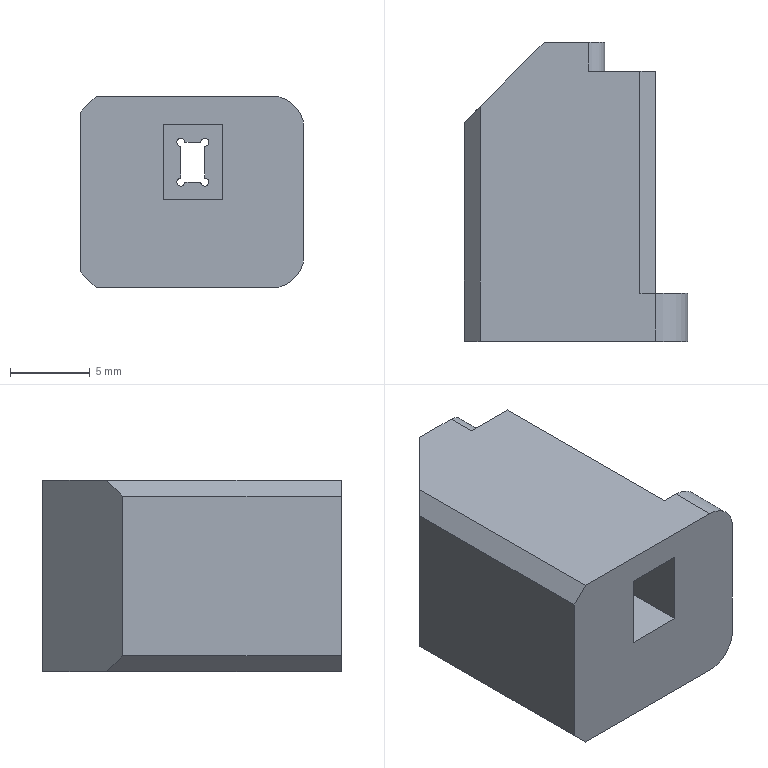Part | STEP file | 03-02 left cutter pad block | 1 solid | 40 faces | box 14 x 18.7 x 12 mm | volume 2273 mm3 | plane 26 | cylinder 14 | commonest cylinder face diameters 0.5 x6 0.6 x4 2 x2 4 x2
STEP:
#1=CARTESIAN_POINT('',(2.4,16.7,-0.58));
#2=VERTEX_POINT('',#1);
#3=CARTESIAN_POINT('',(2.4,16.7,0.02));
#4=VERTEX_POINT('',#3);
#5=CARTESIAN_POINT('',(2.4,16.7,-0.28));
#6=DIRECTION('',(0.,1.,0.));
#7=DIRECTION('',(0.,0.,1.));
#8=AXIS2_PLACEMENT_3D('',#5,#6,#7);
#9=CIRCLE('',#8,0.3);
#10=EDGE_CURVE('',#2,#4,#9,.T.);
#11=ORIENTED_EDGE('',*,*,#10,.F.);
#12=CARTESIAN_POINT('',(2.4,18.7,-0.58));
#13=VERTEX_POINT('',#12);
#14=CARTESIAN_POINT('',(2.4,16.7,-0.58));
#15=DIRECTION('',(0.,1.,0.));
#16=VECTOR('',#15,1000.);
#17=LINE('',#14,#16);
#18=EDGE_CURVE('',#2,#13,#17,.T.);
#19=ORIENTED_EDGE('',*,*,#18,.T.);
#20=CARTESIAN_POINT('',(2.4,18.7,0.02));
#21=VERTEX_POINT('',#20);
#22=CARTESIAN_POINT('',(2.4,18.7,-0.28));
#23=DIRECTION('',(0.,1.,0.));
#24=DIRECTION('',(0.,0.,1.));
#25=AXIS2_PLACEMENT_3D('',#22,#23,#24);
#26=CIRCLE('',#25,0.3);
#27=EDGE_CURVE('',#13,#21,#26,.T.);
#28=ORIENTED_EDGE('',*,*,#27,.T.);
#29=CARTESIAN_POINT('',(2.4,16.7,0.02));
#30=DIRECTION('',(0.,1.,0.));
#31=VECTOR('',#30,1000.);
#32=LINE('',#29,#31);
#33=EDGE_CURVE('',#4,#21,#32,.T.);
#34=ORIENTED_EDGE('',*,*,#33,.F.);
#35=EDGE_LOOP('',(#11,#19,#28,#34));
#36=FACE_OUTER_BOUND('',#35,.T.);
#37=CARTESIAN_POINT('',(2.4,16.7,-0.28));
#38=DIRECTION('',(0.,1.,0.));
#39=DIRECTION('',(0.,0.,1.));
#40=AXIS2_PLACEMENT_3D('',#37,#38,#39);
#41=CYLINDRICAL_SURFACE('',#40,0.3);
#42=ADVANCED_FACE('',(#36),#41,.F.);
#43=CARTESIAN_POINT('',(2.4,16.7,0.62));
#44=VERTEX_POINT('',#43);
#45=CARTESIAN_POINT('',(2.4,16.7,1.22));
#46=VERTEX_POINT('',#45);
#47=CARTESIAN_POINT('',(2.4,16.7,0.92));
#48=DIRECTION('',(0.,1.,0.));
#49=DIRECTION('',(0.,0.,1.));
#50=AXIS2_PLACEMENT_3D('',#47,#48,#49);
#51=CIRCLE('',#50,0.3);
#52=EDGE_CURVE('',#44,#46,#51,.T.);
#53=ORIENTED_EDGE('',*,*,#52,.F.);
#54=CARTESIAN_POINT('',(2.4,18.7,0.62));
#55=VERTEX_POINT('',#54);
#56=CARTESIAN_POINT('',(2.4,16.7,0.62));
#57=DIRECTION('',(0.,1.,0.));
#58=VECTOR('',#57,1000.);
#59=LINE('',#56,#58);
#60=EDGE_CURVE('',#44,#55,#59,.T.);
#61=ORIENTED_EDGE('',*,*,#60,.T.);
#62=CARTESIAN_POINT('',(2.4,18.7,1.22));
#63=VERTEX_POINT('',#62);
#64=CARTESIAN_POINT('',(2.4,18.7,0.92));
#65=DIRECTION('',(0.,1.,0.));
#66=DIRECTION('',(0.,0.,1.));
#67=AXIS2_PLACEMENT_3D('',#64,#65,#66);
#68=CIRCLE('',#67,0.3);
#69=EDGE_CURVE('',#55,#63,#68,.T.);
#70=ORIENTED_EDGE('',*,*,#69,.T.);
#71=CARTESIAN_POINT('',(2.4,16.7,1.22));
#72=DIRECTION('',(0.,1.,0.));
#73=VECTOR('',#72,1000.);
#74=LINE('',#71,#73);
#75=EDGE_CURVE('',#46,#63,#74,.T.);
#76=ORIENTED_EDGE('',*,*,#75,.F.);
#77=EDGE_LOOP('',(#53,#61,#70,#76));
#78=FACE_OUTER_BOUND('',#77,.T.);
#79=CARTESIAN_POINT('',(2.4,16.7,0.92));
#80=DIRECTION('',(0.,1.,0.));
#81=DIRECTION('',(0.,0.,1.));
#82=AXIS2_PLACEMENT_3D('',#79,#80,#81);
#83=CYLINDRICAL_SURFACE('',#82,0.3);
#84=ADVANCED_FACE('',(#78),#83,.F.);
#85=CARTESIAN_POINT('',(1.8,12.,2.87));
#86=VERTEX_POINT('',#85);
#87=CARTESIAN_POINT('',(1.8,12.,3.37));
#88=VERTEX_POINT('',#87);
#89=CARTESIAN_POINT('',(1.8,12.,3.12));
#90=DIRECTION('',(0.,-1.,0.));
#91=DIRECTION('',(0.,0.,-1.));
#92=AXIS2_PLACEMENT_3D('',#89,#90,#91);
#93=CIRCLE('',#92,0.25);
#94=EDGE_CURVE('',#86,#88,#93,.T.);
#95=ORIENTED_EDGE('',*,*,#94,.T.);
#96=CARTESIAN_POINT('',(1.8,18.7,3.37));
#97=VERTEX_POINT('',#96);
#98=CARTESIAN_POINT('',(1.8,8.7,3.37));
#99=DIRECTION('',(0.,1.,0.));
#100=VECTOR('',#99,1000.);
#101=LINE('',#98,#100);
#102=EDGE_CURVE('',#88,#97,#101,.T.);
#103=ORIENTED_EDGE('',*,*,#102,.T.);
#104=CARTESIAN_POINT('',(1.8,18.7,2.87));
#105=VERTEX_POINT('',#104);
#106=CARTESIAN_POINT('',(1.8,18.7,3.12));
#107=DIRECTION('',(0.,1.,0.));
#108=DIRECTION('',(0.,0.,1.));
#109=AXIS2_PLACEMENT_3D('',#106,#107,#108);
#110=CIRCLE('',#109,0.25);
#111=EDGE_CURVE('',#97,#105,#110,.T.);
#112=ORIENTED_EDGE('',*,*,#111,.T.);
#113=CARTESIAN_POINT('',(1.8,8.7,2.87));
#114=DIRECTION('',(0.,1.,0.));
#115=VECTOR('',#114,1000.);
#116=LINE('',#113,#115);
#117=EDGE_CURVE('',#86,#105,#116,.T.);
#118=ORIENTED_EDGE('',*,*,#117,.F.);
#119=EDGE_LOOP('',(#95,#103,#112,#118));
#120=FACE_OUTER_BOUND('',#119,.T.);
#121=CARTESIAN_POINT('',(1.8,8.7,3.12));
#122=DIRECTION('',(0.,1.,0.));
#123=DIRECTION('',(0.,0.,1.));
#124=AXIS2_PLACEMENT_3D('',#121,#122,#123);
#125=CYLINDRICAL_SURFACE('',#124,0.25);
#126=ADVANCED_FACE('',(#120),#125,.F.);
#127=CARTESIAN_POINT('',(0.55,12.,3.12));
#128=VERTEX_POINT('',#127);
#129=CARTESIAN_POINT('',(0.3,12.,3.37));
#130=VERTEX_POINT('',#129);
#131=CARTESIAN_POINT('',(0.3,12.,3.12));
#132=DIRECTION('',(0.,-1.,0.));
#133=DIRECTION('',(0.,0.,-1.));
#134=AXIS2_PLACEMENT_3D('',#131,#132,#133);
#135=CIRCLE('',#134,0.25);
#136=EDGE_CURVE('',#128,#130,#135,.T.);
#137=ORIENTED_EDGE('',*,*,#136,.T.);
#138=CARTESIAN_POINT('',(0.3,18.7,3.37));
#139=VERTEX_POINT('',#138);
#140=CARTESIAN_POINT('',(0.3,8.7,3.37));
#141=DIRECTION('',(0.,1.,0.));
#142=VECTOR('',#141,1000.);
#143=LINE('',#140,#142);
#144=EDGE_CURVE('',#130,#139,#143,.T.);
#145=ORIENTED_EDGE('',*,*,#144,.T.);
#146=CARTESIAN_POINT('',(0.55,18.7,3.12));
#147=VERTEX_POINT('',#146);
#148=CARTESIAN_POINT('',(0.3,18.7,3.12));
#149=DIRECTION('',(0.,1.,0.));
#150=DIRECTION('',(0.,0.,1.));
#151=AXIS2_PLACEMENT_3D('',#148,#149,#150);
#152=CIRCLE('',#151,0.25);
#153=EDGE_CURVE('',#139,#147,#152,.T.);
#154=ORIENTED_EDGE('',*,*,#153,.T.);
#155=CARTESIAN_POINT('',(0.55,8.7,3.12));
#156=DIRECTION('',(0.,1.,0.));
#157=VECTOR('',#156,1000.);
#158=LINE('',#155,#157);
#159=EDGE_CURVE('',#128,#147,#158,.T.);
#160=ORIENTED_EDGE('',*,*,#159,.F.);
#161=EDGE_LOOP('',(#137,#145,#154,#160));
#162=FACE_OUTER_BOUND('',#161,.T.);
#163=CARTESIAN_POINT('',(0.3,8.7,3.12));
#164=DIRECTION('',(0.,1.,0.));
#165=DIRECTION('',(0.,0.,1.));
#166=AXIS2_PLACEMENT_3D('',#163,#164,#165);
#167=CYLINDRICAL_SURFACE('',#166,0.25);
#168=ADVANCED_FACE('',(#162),#167,.F.);
#169=CARTESIAN_POINT('',(0.3,18.7,0.87));
#170=VERTEX_POINT('',#169);
#171=CARTESIAN_POINT('',(0.3,18.7,2.87));
#172=VERTEX_POINT('',#171);
#173=CARTESIAN_POINT('',(0.3,18.7,0.62));
#174=DIRECTION('',(0.,0.,1.));
#175=VECTOR('',#174,1000.);
#176=LINE('',#173,#175);
#177=EDGE_CURVE('',#170,#172,#176,.T.);
#178=ORIENTED_EDGE('',*,*,#177,.T.);
#179=CARTESIAN_POINT('',(0.3,12.,2.87));
#180=VERTEX_POINT('',#179);
#181=CARTESIAN_POINT('',(0.3,8.7,2.87));
#182=DIRECTION('',(0.,-1.,0.));
#183=VECTOR('',#182,1000.);
#184=LINE('',#181,#183);
#185=EDGE_CURVE('',#172,#180,#184,.T.);
#186=ORIENTED_EDGE('',*,*,#185,.T.);
#187=CARTESIAN_POINT('',(0.3,12.,0.87));
#188=VERTEX_POINT('',#187);
#189=CARTESIAN_POINT('',(0.3,12.,0.62));
#190=DIRECTION('',(0.,0.,1.));
#191=VECTOR('',#190,1000.);
#192=LINE('',#189,#191);
#193=EDGE_CURVE('',#188,#180,#192,.T.);
#194=ORIENTED_EDGE('',*,*,#193,.F.);
#195=CARTESIAN_POINT('',(0.3,8.7,0.87));
#196=DIRECTION('',(0.,1.,0.));
#197=VECTOR('',#196,1000.);
#198=LINE('',#195,#197);
#199=EDGE_CURVE('',#188,#170,#198,.T.);
#200=ORIENTED_EDGE('',*,*,#199,.T.);
#201=EDGE_LOOP('',(#178,#186,#194,#200));
#202=FACE_OUTER_BOUND('',#201,.T.);
#203=CARTESIAN_POINT('',(0.3,-11.3,0.62));
#204=DIRECTION('',(-1.,0.,0.));
#205=DIRECTION('',(0.,0.,1.));
#206=AXIS2_PLACEMENT_3D('',#203,#204,#205);
#207=PLANE('',#206);
#208=ADVANCED_FACE('',(#202),#207,.F.);
#209=CARTESIAN_POINT('',(1.55,12.,0.62));
#210=VERTEX_POINT('',#209);
#211=CARTESIAN_POINT('',(0.55,12.,0.62));
#212=VERTEX_POINT('',#211);
#213=CARTESIAN_POINT('',(0.3,12.,0.62));
#214=DIRECTION('',(-1.,0.,0.));
#215=VECTOR('',#214,1000.);
#216=LINE('',#213,#215);
#217=EDGE_CURVE('',#210,#212,#216,.T.);
#218=ORIENTED_EDGE('',*,*,#217,.F.);
#219=CARTESIAN_POINT('',(1.55,18.7,0.62));
#220=VERTEX_POINT('',#219);
#221=CARTESIAN_POINT('',(1.55,8.7,0.62));
#222=DIRECTION('',(0.,1.,0.));
#223=VECTOR('',#222,1000.);
#224=LINE('',#221,#223);
#225=EDGE_CURVE('',#210,#220,#224,.T.);
#226=ORIENTED_EDGE('',*,*,#225,.T.);
#227=CARTESIAN_POINT('',(0.55,18.7,0.62));
#228=VERTEX_POINT('',#227);
#229=CARTESIAN_POINT('',(0.3,18.7,0.62));
#230=DIRECTION('',(-1.,0.,0.));
#231=VECTOR('',#230,1000.);
#232=LINE('',#229,#231);
#233=EDGE_CURVE('',#220,#228,#232,.T.);
#234=ORIENTED_EDGE('',*,*,#233,.T.);
#235=CARTESIAN_POINT('',(0.55,8.7,0.62));
#236=DIRECTION('',(0.,-1.,0.));
#237=VECTOR('',#236,1000.);
#238=LINE('',#235,#237);
#239=EDGE_CURVE('',#228,#212,#238,.T.);
#240=ORIENTED_EDGE('',*,*,#239,.T.);
#241=EDGE_LOOP('',(#218,#226,#234,#240));
#242=FACE_OUTER_BOUND('',#241,.T.);
#243=CARTESIAN_POINT('',(0.3,-11.3,0.62));
#244=DIRECTION('',(0.,0.,-1.));
#245=DIRECTION('',(-1.,0.,0.));
#246=AXIS2_PLACEMENT_3D('',#243,#244,#245);
#247=PLANE('',#246);
#248=ADVANCED_FACE('',(#242),#247,.F.);
#249=CARTESIAN_POINT('',(1.8,12.,0.87));
#250=VERTEX_POINT('',#249);
#251=CARTESIAN_POINT('',(1.8,12.,0.62));
#252=DIRECTION('',(0.,0.,-1.));
#253=VECTOR('',#252,1000.);
#254=LINE('',#251,#253);
#255=EDGE_CURVE('',#86,#250,#254,.T.);
#256=ORIENTED_EDGE('',*,*,#255,.F.);
#257=ORIENTED_EDGE('',*,*,#117,.T.);
#258=CARTESIAN_POINT('',(1.8,18.7,0.87));
#259=VERTEX_POINT('',#258);
#260=CARTESIAN_POINT('',(1.8,18.7,0.62));
#261=DIRECTION('',(0.,0.,-1.));
#262=VECTOR('',#261,1000.);
#263=LINE('',#260,#262);
#264=EDGE_CURVE('',#105,#259,#263,.T.);
#265=ORIENTED_EDGE('',*,*,#264,.T.);
#266=CARTESIAN_POINT('',(1.8,8.7,0.87));
#267=DIRECTION('',(0.,-1.,0.));
#268=VECTOR('',#267,1000.);
#269=LINE('',#266,#268);
#270=EDGE_CURVE('',#259,#250,#269,.T.);
#271=ORIENTED_EDGE('',*,*,#270,.T.);
#272=EDGE_LOOP('',(#256,#257,#265,#271));
#273=FACE_OUTER_BOUND('',#272,.T.);
#274=CARTESIAN_POINT('',(1.8,-11.3,0.62));
#275=DIRECTION('',(1.,0.,0.));
#276=DIRECTION('',(0.,0.,-1.));
#277=AXIS2_PLACEMENT_3D('',#274,#275,#276);
#278=PLANE('',#277);
#279=ADVANCED_FACE('',(#273),#278,.F.);
#280=CARTESIAN_POINT('',(1.55,18.7,3.12));
#281=VERTEX_POINT('',#280);
#282=CARTESIAN_POINT('',(0.3,18.7,3.12));
#283=DIRECTION('',(1.,0.,0.));
#284=VECTOR('',#283,1000.);
#285=LINE('',#282,#284);
#286=EDGE_CURVE('',#147,#281,#285,.T.);
#287=ORIENTED_EDGE('',*,*,#286,.T.);
#288=CARTESIAN_POINT('',(1.55,12.,3.12));
#289=VERTEX_POINT('',#288);
#290=CARTESIAN_POINT('',(1.55,8.7,3.12));
#291=DIRECTION('',(0.,-1.,0.));
#292=VECTOR('',#291,1000.);
#293=LINE('',#290,#292);
#294=EDGE_CURVE('',#281,#289,#293,.T.);
#295=ORIENTED_EDGE('',*,*,#294,.T.);
#296=CARTESIAN_POINT('',(0.3,12.,3.12));
#297=DIRECTION('',(1.,0.,0.));
#298=VECTOR('',#297,1000.);
#299=LINE('',#296,#298);
#300=EDGE_CURVE('',#128,#289,#299,.T.);
#301=ORIENTED_EDGE('',*,*,#300,.F.);
#302=ORIENTED_EDGE('',*,*,#159,.T.);
#303=EDGE_LOOP('',(#287,#295,#301,#302));
#304=FACE_OUTER_BOUND('',#303,.T.);
#305=CARTESIAN_POINT('',(0.3,-11.3,3.12));
#306=DIRECTION('',(0.,0.,1.));
#307=DIRECTION('',(1.,0.,0.));
#308=AXIS2_PLACEMENT_3D('',#305,#306,#307);
#309=PLANE('',#308);
#310=ADVANCED_FACE('',(#304),#309,.F.);
#311=CARTESIAN_POINT('',(6.,3.,-5.));
#312=VERTEX_POINT('',#311);
#313=CARTESIAN_POINT('',(6.,3.,5.));
#314=VERTEX_POINT('',#313);
#315=CARTESIAN_POINT('',(6.,3.,-6.));
#316=DIRECTION('',(0.,0.,1.));
#317=VECTOR('',#316,1000.);
#318=LINE('',#315,#317);
#319=EDGE_CURVE('',#312,#314,#318,.T.);
#320=ORIENTED_EDGE('',*,*,#319,.F.);
#321=CARTESIAN_POINT('',(6.,16.9,-5.));
#322=VERTEX_POINT('',#321);
#323=CARTESIAN_POINT('',(6.,18.7,-5.));
#324=DIRECTION('',(0.,1.,0.));
#325=VECTOR('',#324,1000.);
#326=LINE('',#323,#325);
#327=EDGE_CURVE('',#312,#322,#326,.T.);
#328=ORIENTED_EDGE('',*,*,#327,.T.);
#329=CARTESIAN_POINT('',(6.,16.9,5.));
#330=VERTEX_POINT('',#329);
#331=CARTESIAN_POINT('',(6.,16.9,-6.));
#332=DIRECTION('',(0.,0.,-1.));
#333=VECTOR('',#332,1000.);
#334=LINE('',#331,#333);
#335=EDGE_CURVE('',#330,#322,#334,.T.);
#336=ORIENTED_EDGE('',*,*,#335,.F.);
#337=CARTESIAN_POINT('',(6.,18.7,5.));
#338=DIRECTION('',(0.,-1.,0.));
#339=VECTOR('',#338,1000.);
#340=LINE('',#337,#339);
#341=EDGE_CURVE('',#330,#314,#340,.T.);
#342=ORIENTED_EDGE('',*,*,#341,.T.);
#343=EDGE_LOOP('',(#320,#328,#336,#342));
#344=FACE_OUTER_BOUND('',#343,.T.);
#345=CARTESIAN_POINT('',(6.,18.7,-6.));
#346=DIRECTION('',(-1.,0.,0.));
#347=DIRECTION('',(0.,0.,1.));
#348=AXIS2_PLACEMENT_3D('',#345,#346,#347);
#349=PLANE('',#348);
#350=ADVANCED_FACE('',(#344),#349,.F.);
#351=CARTESIAN_POINT('',(5.,3.,6.));
#352=VERTEX_POINT('',#351);
#353=CARTESIAN_POINT('',(5.,16.9,6.));
#354=VERTEX_POINT('',#353);
#355=CARTESIAN_POINT('',(5.,18.7,6.));
#356=DIRECTION('',(0.,1.,0.));
#357=VECTOR('',#356,1000.);
#358=LINE('',#355,#357);
#359=EDGE_CURVE('',#352,#354,#358,.T.);
#360=ORIENTED_EDGE('',*,*,#359,.F.);
#361=CARTESIAN_POINT('',(6.,3.,5.));
#362=DIRECTION('',(0.7071,0.,-0.7071));
#363=VECTOR('',#362,1000.);
#364=LINE('',#361,#363);
#365=EDGE_CURVE('',#352,#314,#364,.T.);
#366=ORIENTED_EDGE('',*,*,#365,.T.);
#367=ORIENTED_EDGE('',*,*,#341,.F.);
#368=CARTESIAN_POINT('',(3.627,16.9,7.373));
#369=DIRECTION('',(0.7071,0.,-0.7071));
#370=VECTOR('',#369,1000.);
#371=LINE('',#368,#370);
#372=EDGE_CURVE('',#354,#330,#371,.T.);
#373=ORIENTED_EDGE('',*,*,#372,.F.);
#374=EDGE_LOOP('',(#360,#366,#367,#373));
#375=FACE_OUTER_BOUND('',#374,.T.);
#376=CARTESIAN_POINT('',(6.,18.7,5.));
#377=DIRECTION('',(-0.7071,0.,-0.7071));
#378=DIRECTION('',(-0.7071,0.,0.7071));
#379=AXIS2_PLACEMENT_3D('',#376,#377,#378);
#380=PLANE('',#379);
#381=ADVANCED_FACE('',(#375),#380,.F.);
#382=ORIENTED_EDGE('',*,*,#327,.F.);
#383=CARTESIAN_POINT('',(5.,3.,-6.));
#384=VERTEX_POINT('',#383);
#385=CARTESIAN_POINT('',(5.,3.,-6.));
#386=DIRECTION('',(-0.7071,0.,-0.7071));
#387=VECTOR('',#386,1000.);
#388=LINE('',#385,#387);
#389=EDGE_CURVE('',#312,#384,#388,.T.);
#390=ORIENTED_EDGE('',*,*,#389,.T.);
#391=CARTESIAN_POINT('',(5.,16.9,-6.));
#392=VERTEX_POINT('',#391);
#393=CARTESIAN_POINT('',(5.,18.7,-6.));
#394=DIRECTION('',(0.,-1.,0.));
#395=VECTOR('',#394,1000.);
#396=LINE('',#393,#395);
#397=EDGE_CURVE('',#392,#384,#396,.T.);
#398=ORIENTED_EDGE('',*,*,#397,.F.);
#399=CARTESIAN_POINT('',(10.173,16.9,-0.8274));
#400=DIRECTION('',(-0.7071,0.,-0.7071));
#401=VECTOR('',#400,1000.);
#402=LINE('',#399,#401);
#403=EDGE_CURVE('',#322,#392,#402,.T.);
#404=ORIENTED_EDGE('',*,*,#403,.F.);
#405=EDGE_LOOP('',(#382,#390,#398,#404));
#406=FACE_OUTER_BOUND('',#405,.T.);
#407=CARTESIAN_POINT('',(5.,18.7,-6.));
#408=DIRECTION('',(-0.7071,0.,0.7071));
#409=DIRECTION('',(0.7071,0.,0.7071));
#410=AXIS2_PLACEMENT_3D('',#407,#408,#409);
#411=PLANE('',#410);
#412=ADVANCED_FACE('',(#406),#411,.F.);
#413=CARTESIAN_POINT('',(6.,3.,-6.));
#414=VERTEX_POINT('',#413);
#415=CARTESIAN_POINT('',(5.,3.,-6.));
#416=DIRECTION('',(1.,0.,0.));
#417=VECTOR('',#416,1000.);
#418=LINE('',#415,#417);
#419=EDGE_CURVE('',#384,#414,#418,.T.);
#420=ORIENTED_EDGE('',*,*,#419,.T.);
#421=CARTESIAN_POINT('',(6.,0.,-6.));
#422=VERTEX_POINT('',#421);
#423=CARTESIAN_POINT('',(6.,0.,-6.));
#424=DIRECTION('',(0.,-1.,0.));
#425=VECTOR('',#424,1000.);
#426=LINE('',#423,#425);
#427=EDGE_CURVE('',#414,#422,#426,.T.);
#428=ORIENTED_EDGE('',*,*,#427,.T.);
#429=CARTESIAN_POINT('',(-5.,0.,-6.));
#430=VERTEX_POINT('',#429);
#431=CARTESIAN_POINT('',(-6.,0.,-6.));
#432=DIRECTION('',(-1.,0.,0.));
#433=VECTOR('',#432,1000.);
#434=LINE('',#431,#433);
#435=EDGE_CURVE('',#422,#430,#434,.T.);
#436=ORIENTED_EDGE('',*,*,#435,.T.);
#437=CARTESIAN_POINT('',(-5.,14.7,-6.));
#438=VERTEX_POINT('',#437);
#439=CARTESIAN_POINT('',(-5.,18.7,-6.));
#440=DIRECTION('',(0.,1.,0.));
#441=VECTOR('',#440,1000.);
#442=LINE('',#439,#441);
#443=EDGE_CURVE('',#430,#438,#442,.T.);
#444=ORIENTED_EDGE('',*,*,#443,.T.);
#445=CARTESIAN_POINT('',(-1.,18.7,-6.));
#446=VERTEX_POINT('',#445);
#447=CARTESIAN_POINT('',(-1.,18.7,-6.));
#448=DIRECTION('',(0.7071,0.7071,0.));
#449=VECTOR('',#448,1000.);
#450=LINE('',#447,#449);
#451=EDGE_CURVE('',#438,#446,#450,.T.);
#452=ORIENTED_EDGE('',*,*,#451,.T.);
#453=CARTESIAN_POINT('',(1.8,18.7,-6.));
#454=VERTEX_POINT('',#453);
#455=CARTESIAN_POINT('',(-6.,18.7,-6.));
#456=DIRECTION('',(-1.,0.,0.));
#457=VECTOR('',#456,1000.);
#458=LINE('',#455,#457);
#459=EDGE_CURVE('',#454,#446,#458,.T.);
#460=ORIENTED_EDGE('',*,*,#459,.F.);
#461=CARTESIAN_POINT('',(1.8,16.9,-6.));
#462=VERTEX_POINT('',#461);
#463=CARTESIAN_POINT('',(1.8,18.7,-6.));
#464=DIRECTION('',(0.,-1.,0.));
#465=VECTOR('',#464,1000.);
#466=LINE('',#463,#465);
#467=EDGE_CURVE('',#454,#462,#466,.T.);
#468=ORIENTED_EDGE('',*,*,#467,.T.);
#469=CARTESIAN_POINT('',(-6.,16.9,-6.));
#470=DIRECTION('',(-1.,0.,0.));
#471=VECTOR('',#470,1000.);
#472=LINE('',#469,#471);
#473=EDGE_CURVE('',#392,#462,#472,.T.);
#474=ORIENTED_EDGE('',*,*,#473,.F.);
#475=ORIENTED_EDGE('',*,*,#397,.T.);
#476=EDGE_LOOP('',(#420,#428,#436,#444,#452,#460,#468,#474,#475));
#477=FACE_OUTER_BOUND('',#476,.T.);
#478=CARTESIAN_POINT('',(-6.,18.7,-6.));
#479=DIRECTION('',(0.,0.,1.));
#480=DIRECTION('',(1.,0.,0.));
#481=AXIS2_PLACEMENT_3D('',#478,#479,#480);
#482=PLANE('',#481);
#483=ADVANCED_FACE('',(#477),#482,.F.);
#484=CARTESIAN_POINT('',(-6.,0.,5.));
#485=VERTEX_POINT('',#484);
#486=CARTESIAN_POINT('',(-6.,13.7,5.));
#487=VERTEX_POINT('',#486);
#488=CARTESIAN_POINT('',(-6.,18.7,5.));
#489=DIRECTION('',(0.,1.,0.));
#490=VECTOR('',#489,1000.);
#491=LINE('',#488,#490);
#492=EDGE_CURVE('',#485,#487,#491,.T.);
#493=ORIENTED_EDGE('',*,*,#492,.T.);
#494=CARTESIAN_POINT('',(-6.,13.7,-5.));
#495=VERTEX_POINT('',#494);
#496=CARTESIAN_POINT('',(-6.,13.7,-5.));
#497=DIRECTION('',(0.,0.,-1.));
#498=VECTOR('',#497,1000.);
#499=LINE('',#496,#498);
#500=EDGE_CURVE('',#487,#495,#499,.T.);
#501=ORIENTED_EDGE('',*,*,#500,.T.);
#502=CARTESIAN_POINT('',(-6.,0.,-5.));
#503=VERTEX_POINT('',#502);
#504=CARTESIAN_POINT('',(-6.,18.7,-5.));
#505=DIRECTION('',(0.,-1.,0.));
#506=VECTOR('',#505,1000.);
#507=LINE('',#504,#506);
#508=EDGE_CURVE('',#495,#503,#507,.T.);
#509=ORIENTED_EDGE('',*,*,#508,.T.);
#510=CARTESIAN_POINT('',(-6.,0.,-6.));
#511=DIRECTION('',(0.,0.,1.));
#512=VECTOR('',#511,1000.);
#513=LINE('',#510,#512);
#514=EDGE_CURVE('',#503,#485,#513,.T.);
#515=ORIENTED_EDGE('',*,*,#514,.T.);
#516=EDGE_LOOP('',(#493,#501,#509,#515));
#517=FACE_OUTER_BOUND('',#516,.T.);
#518=CARTESIAN_POINT('',(-6.,18.7,-6.));
#519=DIRECTION('',(1.,0.,0.));
#520=DIRECTION('',(0.,0.,-1.));
#521=AXIS2_PLACEMENT_3D('',#518,#519,#520);
#522=PLANE('',#521);
#523=ADVANCED_FACE('',(#517),#522,.F.);
#524=CARTESIAN_POINT('',(-5.,0.,6.));
#525=VERTEX_POINT('',#524);
#526=CARTESIAN_POINT('',(6.,0.,6.));
#527=VERTEX_POINT('',#526);
#528=CARTESIAN_POINT('',(-6.,0.,6.));
#529=DIRECTION('',(1.,0.,0.));
#530=VECTOR('',#529,1000.);
#531=LINE('',#528,#530);
#532=EDGE_CURVE('',#525,#527,#531,.T.);
#533=ORIENTED_EDGE('',*,*,#532,.T.);
#534=CARTESIAN_POINT('',(6.,3.,6.));
#535=VERTEX_POINT('',#534);
#536=CARTESIAN_POINT('',(6.,3.,6.));
#537=DIRECTION('',(0.,1.,0.));
#538=VECTOR('',#537,1000.);
#539=LINE('',#536,#538);
#540=EDGE_CURVE('',#527,#535,#539,.T.);
#541=ORIENTED_EDGE('',*,*,#540,.T.);
#542=CARTESIAN_POINT('',(5.,3.,6.));
#543=DIRECTION('',(-1.,0.,0.));
#544=VECTOR('',#543,1000.);
#545=LINE('',#542,#544);
#546=EDGE_CURVE('',#535,#352,#545,.T.);
#547=ORIENTED_EDGE('',*,*,#546,.T.);
#548=ORIENTED_EDGE('',*,*,#359,.T.);
#549=CARTESIAN_POINT('',(1.8,16.9,6.));
#550=VERTEX_POINT('',#549);
#551=CARTESIAN_POINT('',(-6.,16.9,6.));
#552=DIRECTION('',(1.,0.,0.));
#553=VECTOR('',#552,1000.);
#554=LINE('',#551,#553);
#555=EDGE_CURVE('',#550,#354,#554,.T.);
#556=ORIENTED_EDGE('',*,*,#555,.F.);
#557=CARTESIAN_POINT('',(1.8,18.7,6.));
#558=VERTEX_POINT('',#557);
#559=CARTESIAN_POINT('',(1.8,18.7,6.));
#560=DIRECTION('',(0.,1.,0.));
#561=VECTOR('',#560,1000.);
#562=LINE('',#559,#561);
#563=EDGE_CURVE('',#550,#558,#562,.T.);
#564=ORIENTED_EDGE('',*,*,#563,.T.);
#565=CARTESIAN_POINT('',(-1.,18.7,6.));
#566=VERTEX_POINT('',#565);
#567=CARTESIAN_POINT('',(-6.,18.7,6.));
#568=DIRECTION('',(1.,0.,0.));
#569=VECTOR('',#568,1000.);
#570=LINE('',#567,#569);
#571=EDGE_CURVE('',#566,#558,#570,.T.);
#572=ORIENTED_EDGE('',*,*,#571,.F.);
#573=CARTESIAN_POINT('',(-5.,14.7,6.));
#574=VERTEX_POINT('',#573);
#575=CARTESIAN_POINT('',(-1.,18.7,6.));
#576=DIRECTION('',(-0.7071,-0.7071,0.));
#577=VECTOR('',#576,1000.);
#578=LINE('',#575,#577);
#579=EDGE_CURVE('',#566,#574,#578,.T.);
#580=ORIENTED_EDGE('',*,*,#579,.T.);
#581=CARTESIAN_POINT('',(-5.,18.7,6.));
#582=DIRECTION('',(0.,-1.,0.));
#583=VECTOR('',#582,1000.);
#584=LINE('',#581,#583);
#585=EDGE_CURVE('',#574,#525,#584,.T.);
#586=ORIENTED_EDGE('',*,*,#585,.T.);
#587=EDGE_LOOP('',(#533,#541,#547,#548,#556,#564,#572,#580,#586));
#588=FACE_OUTER_BOUND('',#587,.T.);
#589=CARTESIAN_POINT('',(-6.,18.7,6.));
#590=DIRECTION('',(0.,0.,-1.));
#591=DIRECTION('',(-1.,0.,0.));
#592=AXIS2_PLACEMENT_3D('',#589,#590,#591);
#593=PLANE('',#592);
#594=ADVANCED_FACE('',(#588),#593,.F.);
#595=CARTESIAN_POINT('',(2.4,18.7,-0.28));
#596=DIRECTION('',(0.,1.,0.));
#597=DIRECTION('',(0.,0.,1.));
#598=AXIS2_PLACEMENT_3D('',#595,#596,#597);
#599=CIRCLE('',#598,0.3);
#600=EDGE_CURVE('',#21,#13,#599,.T.);
#601=ORIENTED_EDGE('',*,*,#600,.F.);
#602=ORIENTED_EDGE('',*,*,#27,.F.);
#603=EDGE_LOOP('',(#601,#602));
#604=FACE_BOUND('',#603,.T.);
#605=CARTESIAN_POINT('',(2.4,18.7,0.92));
#606=DIRECTION('',(0.,1.,0.));
#607=DIRECTION('',(0.,0.,1.));
#608=AXIS2_PLACEMENT_3D('',#605,#606,#607);
#609=CIRCLE('',#608,0.3);
#610=EDGE_CURVE('',#63,#55,#609,.T.);
#611=ORIENTED_EDGE('',*,*,#610,.F.);
#612=ORIENTED_EDGE('',*,*,#69,.F.);
#613=EDGE_LOOP('',(#611,#612));
#614=FACE_BOUND('',#613,.T.);
#615=CARTESIAN_POINT('',(1.8,18.7,3.12));
#616=DIRECTION('',(0.,1.,0.));
#617=DIRECTION('',(0.,0.,1.));
#618=AXIS2_PLACEMENT_3D('',#615,#616,#617);
#619=CIRCLE('',#618,0.25);
#620=EDGE_CURVE('',#281,#97,#619,.T.);
#621=ORIENTED_EDGE('',*,*,#620,.F.);
#622=ORIENTED_EDGE('',*,*,#286,.F.);
#623=ORIENTED_EDGE('',*,*,#153,.F.);
#624=CARTESIAN_POINT('',(0.3,18.7,3.12));
#625=DIRECTION('',(0.,1.,0.));
#626=DIRECTION('',(0.,0.,1.));
#627=AXIS2_PLACEMENT_3D('',#624,#625,#626);
#628=CIRCLE('',#627,0.25);
#629=EDGE_CURVE('',#172,#139,#628,.T.);
#630=ORIENTED_EDGE('',*,*,#629,.F.);
#631=ORIENTED_EDGE('',*,*,#177,.F.);
#632=CARTESIAN_POINT('',(0.3,18.7,0.62));
#633=DIRECTION('',(0.,1.,0.));
#634=DIRECTION('',(0.,0.,1.));
#635=AXIS2_PLACEMENT_3D('',#632,#633,#634);
#636=CIRCLE('',#635,0.25);
#637=EDGE_CURVE('',#228,#170,#636,.T.);
#638=ORIENTED_EDGE('',*,*,#637,.F.);
#639=ORIENTED_EDGE('',*,*,#233,.F.);
#640=CARTESIAN_POINT('',(1.8,18.7,0.62));
#641=DIRECTION('',(0.,1.,0.));
#642=DIRECTION('',(0.,0.,1.));
#643=AXIS2_PLACEMENT_3D('',#640,#641,#642);
#644=CIRCLE('',#643,0.25);
#645=EDGE_CURVE('',#259,#220,#644,.T.);
#646=ORIENTED_EDGE('',*,*,#645,.F.);
#647=ORIENTED_EDGE('',*,*,#264,.F.);
#648=ORIENTED_EDGE('',*,*,#111,.F.);
#649=EDGE_LOOP('',(#621,#622,#623,#630,#631,#638,#639,#646,#647,#648));
#650=FACE_BOUND('',#649,.T.);
#651=ORIENTED_EDGE('',*,*,#459,.T.);
#652=CARTESIAN_POINT('',(-1.,18.7,5.));
#653=DIRECTION('',(0.,0.,1.));
#654=VECTOR('',#653,1000.);
#655=LINE('',#652,#654);
#656=EDGE_CURVE('',#446,#566,#655,.T.);
#657=ORIENTED_EDGE('',*,*,#656,.T.);
#658=ORIENTED_EDGE('',*,*,#571,.T.);
#659=CARTESIAN_POINT('',(2.8,18.7,5.));
#660=VERTEX_POINT('',#659);
#661=CARTESIAN_POINT('',(1.8,18.7,5.));
#662=DIRECTION('',(0.,1.,0.));
#663=DIRECTION('',(0.,0.,1.));
#664=AXIS2_PLACEMENT_3D('',#661,#662,#663);
#665=CIRCLE('',#664,1.);
#666=EDGE_CURVE('',#558,#660,#665,.T.);
#667=ORIENTED_EDGE('',*,*,#666,.T.);
#668=CARTESIAN_POINT('',(2.8,18.7,-5.));
#669=VERTEX_POINT('',#668);
#670=CARTESIAN_POINT('',(2.8,18.7,6.));
#671=DIRECTION('',(0.,0.,1.));
#672=VECTOR('',#671,1000.);
#673=LINE('',#670,#672);
#674=EDGE_CURVE('',#669,#660,#673,.T.);
#675=ORIENTED_EDGE('',*,*,#674,.F.);
#676=CARTESIAN_POINT('',(1.8,18.7,-5.));
#677=DIRECTION('',(0.,1.,0.));
#678=DIRECTION('',(0.,0.,1.));
#679=AXIS2_PLACEMENT_3D('',#676,#677,#678);
#680=CIRCLE('',#679,1.);
#681=EDGE_CURVE('',#669,#454,#680,.T.);
#682=ORIENTED_EDGE('',*,*,#681,.T.);
#683=EDGE_LOOP('',(#651,#657,#658,#667,#675,#682));
#684=FACE_OUTER_BOUND('',#683,.T.);
#685=CARTESIAN_POINT('',(6.,18.7,6.));
#686=DIRECTION('',(0.,1.,0.));
#687=DIRECTION('',(0.,0.,1.));
#688=AXIS2_PLACEMENT_3D('',#685,#686,#687);
#689=PLANE('',#688);
#690=ADVANCED_FACE('',(#604,#614,#650,#684),#689,.T.);
#691=CARTESIAN_POINT('',(-0.8,0.,-0.48));
#692=VERTEX_POINT('',#691);
#693=CARTESIAN_POINT('',(2.9,0.,-0.48));
#694=VERTEX_POINT('',#693);
#695=CARTESIAN_POINT('',(-0.8,0.,-0.48));
#696=DIRECTION('',(1.,0.,0.));
#697=VECTOR('',#696,1000.);
#698=LINE('',#695,#697);
#699=EDGE_CURVE('',#692,#694,#698,.T.);
#700=ORIENTED_EDGE('',*,*,#699,.F.);
#701=CARTESIAN_POINT('',(-0.8,0.,4.22));
#702=VERTEX_POINT('',#701);
#703=CARTESIAN_POINT('',(-0.8,0.,4.22));
#704=DIRECTION('',(0.,0.,-1.));
#705=VECTOR('',#704,1000.);
#706=LINE('',#703,#705);
#707=EDGE_CURVE('',#702,#692,#706,.T.);
#708=ORIENTED_EDGE('',*,*,#707,.F.);
#709=CARTESIAN_POINT('',(2.9,0.,4.22));
#710=VERTEX_POINT('',#709);
#711=CARTESIAN_POINT('',(-0.8,0.,4.22));
#712=DIRECTION('',(-1.,0.,0.));
#713=VECTOR('',#712,1000.);
#714=LINE('',#711,#713);
#715=EDGE_CURVE('',#710,#702,#714,.T.);
#716=ORIENTED_EDGE('',*,*,#715,.F.);
#717=CARTESIAN_POINT('',(2.9,0.,4.22));
#718=DIRECTION('',(0.,0.,1.));
#719=VECTOR('',#718,1000.);
#720=LINE('',#717,#719);
#721=EDGE_CURVE('',#694,#710,#720,.T.);
#722=ORIENTED_EDGE('',*,*,#721,.F.);
#723=EDGE_LOOP('',(#700,#708,#716,#722));
#724=FACE_BOUND('',#723,.T.);
#725=CARTESIAN_POINT('',(8.,0.,-4.));
#726=VERTEX_POINT('',#725);
#727=CARTESIAN_POINT('',(8.,0.,4.));
#728=VERTEX_POINT('',#727);
#729=CARTESIAN_POINT('',(8.,0.,6.));
#730=DIRECTION('',(0.,0.,1.));
#731=VECTOR('',#730,1000.);
#732=LINE('',#729,#731);
#733=EDGE_CURVE('',#726,#728,#732,.T.);
#734=ORIENTED_EDGE('',*,*,#733,.T.);
#735=CARTESIAN_POINT('',(6.,0.,4.));
#736=DIRECTION('',(0.,-1.,0.));
#737=DIRECTION('',(0.,0.,1.));
#738=AXIS2_PLACEMENT_3D('',#735,#736,#737);
#739=CIRCLE('',#738,2.);
#740=EDGE_CURVE('',#728,#527,#739,.T.);
#741=ORIENTED_EDGE('',*,*,#740,.T.);
#742=ORIENTED_EDGE('',*,*,#532,.F.);
#743=CARTESIAN_POINT('',(-5.,0.,6.));
#744=DIRECTION('',(-0.7071,0.,-0.7071));
#745=VECTOR('',#744,1000.);
#746=LINE('',#743,#745);
#747=EDGE_CURVE('',#525,#485,#746,.T.);
#748=ORIENTED_EDGE('',*,*,#747,.T.);
#749=ORIENTED_EDGE('',*,*,#514,.F.);
#750=CARTESIAN_POINT('',(-6.,0.,-5.));
#751=DIRECTION('',(0.7071,0.,-0.7071));
#752=VECTOR('',#751,1000.);
#753=LINE('',#750,#752);
#754=EDGE_CURVE('',#503,#430,#753,.T.);
#755=ORIENTED_EDGE('',*,*,#754,.T.);
#756=ORIENTED_EDGE('',*,*,#435,.F.);
#757=CARTESIAN_POINT('',(6.,0.,-4.));
#758=DIRECTION('',(0.,-1.,0.));
#759=DIRECTION('',(0.,0.,1.));
#760=AXIS2_PLACEMENT_3D('',#757,#758,#759);
#761=CIRCLE('',#760,2.);
#762=EDGE_CURVE('',#422,#726,#761,.T.);
#763=ORIENTED_EDGE('',*,*,#762,.T.);
#764=EDGE_LOOP('',(#734,#741,#742,#748,#749,#755,#756,#763));
#765=FACE_OUTER_BOUND('',#764,.T.);
#766=CARTESIAN_POINT('',(6.,0.,6.));
#767=DIRECTION('',(0.,1.,0.));
#768=DIRECTION('',(0.,0.,1.));
#769=AXIS2_PLACEMENT_3D('',#766,#767,#768);
#770=PLANE('',#769);
#771=ADVANCED_FACE('',(#724,#765),#770,.F.);
#772=ORIENTED_EDGE('',*,*,#555,.T.);
#773=ORIENTED_EDGE('',*,*,#372,.T.);
#774=ORIENTED_EDGE('',*,*,#335,.T.);
#775=ORIENTED_EDGE('',*,*,#403,.T.);
#776=ORIENTED_EDGE('',*,*,#473,.T.);
#777=CARTESIAN_POINT('',(2.8,16.9,-5.));
#778=VERTEX_POINT('',#777);
#779=CARTESIAN_POINT('',(1.8,16.9,-5.));
#780=DIRECTION('',(0.,-1.,0.));
#781=DIRECTION('',(0.,0.,1.));
#782=AXIS2_PLACEMENT_3D('',#779,#780,#781);
#783=CIRCLE('',#782,1.);
#784=EDGE_CURVE('',#462,#778,#783,.T.);
#785=ORIENTED_EDGE('',*,*,#784,.T.);
#786=CARTESIAN_POINT('',(2.8,16.9,5.));
#787=VERTEX_POINT('',#786);
#788=CARTESIAN_POINT('',(2.8,16.9,-6.741));
#789=DIRECTION('',(0.,0.,1.));
#790=VECTOR('',#789,1000.);
#791=LINE('',#788,#790);
#792=EDGE_CURVE('',#778,#787,#791,.T.);
#793=ORIENTED_EDGE('',*,*,#792,.T.);
#794=CARTESIAN_POINT('',(1.8,16.9,5.));
#795=DIRECTION('',(0.,-1.,0.));
#796=DIRECTION('',(0.,0.,1.));
#797=AXIS2_PLACEMENT_3D('',#794,#795,#796);
#798=CIRCLE('',#797,1.);
#799=EDGE_CURVE('',#787,#550,#798,.T.);
#800=ORIENTED_EDGE('',*,*,#799,.T.);
#801=EDGE_LOOP('',(#772,#773,#774,#775,#776,#785,#793,#800));
#802=FACE_OUTER_BOUND('',#801,.T.);
#803=CARTESIAN_POINT('',(2.8,16.9,6.545));
#804=DIRECTION('',(0.,1.,0.));
#805=DIRECTION('',(0.,0.,1.));
#806=AXIS2_PLACEMENT_3D('',#803,#804,#805);
#807=PLANE('',#806);
#808=ADVANCED_FACE('',(#802),#807,.T.);
#809=ORIENTED_EDGE('',*,*,#792,.F.);
#810=CARTESIAN_POINT('',(2.8,16.9,-5.));
#811=DIRECTION('',(0.,1.,0.));
#812=VECTOR('',#811,1000.);
#813=LINE('',#810,#812);
#814=EDGE_CURVE('',#778,#669,#813,.T.);
#815=ORIENTED_EDGE('',*,*,#814,.T.);
#816=ORIENTED_EDGE('',*,*,#674,.T.);
#817=CARTESIAN_POINT('',(2.8,16.9,5.));
#818=DIRECTION('',(0.,-1.,0.));
#819=VECTOR('',#818,1000.);
#820=LINE('',#817,#819);
#821=EDGE_CURVE('',#660,#787,#820,.T.);
#822=ORIENTED_EDGE('',*,*,#821,.T.);
#823=EDGE_LOOP('',(#809,#815,#816,#822));
#824=FACE_OUTER_BOUND('',#823,.T.);
#825=CARTESIAN_POINT('',(2.8,16.9,-6.741));
#826=DIRECTION('',(-1.,0.,0.));
#827=DIRECTION('',(0.,0.,1.));
#828=AXIS2_PLACEMENT_3D('',#825,#826,#827);
#829=PLANE('',#828);
#830=ADVANCED_FACE('',(#824),#829,.F.);
#831=ORIENTED_EDGE('',*,*,#681,.F.);
#832=ORIENTED_EDGE('',*,*,#814,.F.);
#833=ORIENTED_EDGE('',*,*,#784,.F.);
#834=ORIENTED_EDGE('',*,*,#467,.F.);
#835=EDGE_LOOP('',(#831,#832,#833,#834));
#836=FACE_OUTER_BOUND('',#835,.T.);
#837=CARTESIAN_POINT('',(1.8,18.7,-5.));
#838=DIRECTION('',(0.,-1.,0.));
#839=DIRECTION('',(0.,0.,-1.));
#840=AXIS2_PLACEMENT_3D('',#837,#838,#839);
#841=CYLINDRICAL_SURFACE('',#840,1.);
#842=ADVANCED_FACE('',(#836),#841,.T.);
#843=ORIENTED_EDGE('',*,*,#799,.F.);
#844=ORIENTED_EDGE('',*,*,#821,.F.);
#845=ORIENTED_EDGE('',*,*,#666,.F.);
#846=ORIENTED_EDGE('',*,*,#563,.F.);
#847=EDGE_LOOP('',(#843,#844,#845,#846));
#848=FACE_OUTER_BOUND('',#847,.T.);
#849=CARTESIAN_POINT('',(1.8,18.7,5.));
#850=DIRECTION('',(0.,1.,0.));
#851=DIRECTION('',(0.,0.,1.));
#852=AXIS2_PLACEMENT_3D('',#849,#850,#851);
#853=CYLINDRICAL_SURFACE('',#852,1.);
#854=ADVANCED_FACE('',(#848),#853,.T.);
#855=ORIENTED_EDGE('',*,*,#508,.F.);
#856=CARTESIAN_POINT('',(-4.333,15.367,-6.667));
#857=DIRECTION('',(0.5774,0.5774,-0.5774));
#858=VECTOR('',#857,1000.);
#859=LINE('',#856,#858);
#860=EDGE_CURVE('',#495,#438,#859,.T.);
#861=ORIENTED_EDGE('',*,*,#860,.T.);
#862=ORIENTED_EDGE('',*,*,#443,.F.);
#863=ORIENTED_EDGE('',*,*,#754,.F.);
#864=EDGE_LOOP('',(#855,#861,#862,#863));
#865=FACE_OUTER_BOUND('',#864,.T.);
#866=CARTESIAN_POINT('',(-6.,18.7,-5.));
#867=DIRECTION('',(0.7071,0.,0.7071));
#868=DIRECTION('',(0.7071,0.,-0.7071));
#869=AXIS2_PLACEMENT_3D('',#866,#867,#868);
#870=PLANE('',#869);
#871=ADVANCED_FACE('',(#865),#870,.F.);
#872=ORIENTED_EDGE('',*,*,#585,.F.);
#873=CARTESIAN_POINT('',(-3.667,16.033,7.333));
#874=DIRECTION('',(-0.5774,-0.5774,-0.5774));
#875=VECTOR('',#874,1000.);
#876=LINE('',#873,#875);
#877=EDGE_CURVE('',#574,#487,#876,.T.);
#878=ORIENTED_EDGE('',*,*,#877,.T.);
#879=ORIENTED_EDGE('',*,*,#492,.F.);
#880=ORIENTED_EDGE('',*,*,#747,.F.);
#881=EDGE_LOOP('',(#872,#878,#879,#880));
#882=FACE_OUTER_BOUND('',#881,.T.);
#883=CARTESIAN_POINT('',(-5.,18.7,6.));
#884=DIRECTION('',(0.7071,0.,-0.7071));
#885=DIRECTION('',(-0.7071,0.,-0.7071));
#886=AXIS2_PLACEMENT_3D('',#883,#884,#885);
#887=PLANE('',#886);
#888=ADVANCED_FACE('',(#882),#887,.F.);
#889=ORIENTED_EDGE('',*,*,#860,.F.);
#890=ORIENTED_EDGE('',*,*,#500,.F.);
#891=ORIENTED_EDGE('',*,*,#877,.F.);
#892=ORIENTED_EDGE('',*,*,#579,.F.);
#893=ORIENTED_EDGE('',*,*,#656,.F.);
#894=ORIENTED_EDGE('',*,*,#451,.F.);
#895=EDGE_LOOP('',(#889,#890,#891,#892,#893,#894));
#896=FACE_OUTER_BOUND('',#895,.T.);
#897=CARTESIAN_POINT('',(-1.,18.7,6.));
#898=DIRECTION('',(-0.7071,0.7071,0.));
#899=DIRECTION('',(-0.7071,-0.7071,0.));
#900=AXIS2_PLACEMENT_3D('',#897,#898,#899);
#901=PLANE('',#900);
#902=ADVANCED_FACE('',(#896),#901,.T.);
#903=CARTESIAN_POINT('',(8.,3.,-4.));
#904=VERTEX_POINT('',#903);
#905=CARTESIAN_POINT('',(8.,3.,4.));
#906=VERTEX_POINT('',#905);
#907=CARTESIAN_POINT('',(8.,3.,6.));
#908=DIRECTION('',(0.,0.,1.));
#909=VECTOR('',#908,1000.);
#910=LINE('',#907,#909);
#911=EDGE_CURVE('',#904,#906,#910,.T.);
#912=ORIENTED_EDGE('',*,*,#911,.T.);
#913=CARTESIAN_POINT('',(8.,0.,4.));
#914=DIRECTION('',(0.,-1.,0.));
#915=VECTOR('',#914,1000.);
#916=LINE('',#913,#915);
#917=EDGE_CURVE('',#906,#728,#916,.T.);
#918=ORIENTED_EDGE('',*,*,#917,.T.);
#919=ORIENTED_EDGE('',*,*,#733,.F.);
#920=CARTESIAN_POINT('',(8.,3.,-4.));
#921=DIRECTION('',(0.,1.,0.));
#922=VECTOR('',#921,1000.);
#923=LINE('',#920,#922);
#924=EDGE_CURVE('',#726,#904,#923,.T.);
#925=ORIENTED_EDGE('',*,*,#924,.T.);
#926=EDGE_LOOP('',(#912,#918,#919,#925));
#927=FACE_OUTER_BOUND('',#926,.T.);
#928=CARTESIAN_POINT('',(8.,3.,6.));
#929=DIRECTION('',(1.,0.,0.));
#930=DIRECTION('',(0.,0.,-1.));
#931=AXIS2_PLACEMENT_3D('',#928,#929,#930);
#932=PLANE('',#931);
#933=ADVANCED_FACE('',(#927),#932,.T.);
#934=ORIENTED_EDGE('',*,*,#546,.F.);
#935=CARTESIAN_POINT('',(6.,3.,4.));
#936=DIRECTION('',(0.,1.,0.));
#937=DIRECTION('',(0.,0.,-1.));
#938=AXIS2_PLACEMENT_3D('',#935,#936,#937);
#939=CIRCLE('',#938,2.);
#940=EDGE_CURVE('',#535,#906,#939,.T.);
#941=ORIENTED_EDGE('',*,*,#940,.T.);
#942=ORIENTED_EDGE('',*,*,#911,.F.);
#943=CARTESIAN_POINT('',(6.,3.,-4.));
#944=DIRECTION('',(0.,1.,0.));
#945=DIRECTION('',(0.,0.,-1.));
#946=AXIS2_PLACEMENT_3D('',#943,#944,#945);
#947=CIRCLE('',#946,2.);
#948=EDGE_CURVE('',#904,#414,#947,.T.);
#949=ORIENTED_EDGE('',*,*,#948,.T.);
#950=ORIENTED_EDGE('',*,*,#419,.F.);
#951=ORIENTED_EDGE('',*,*,#389,.F.);
#952=ORIENTED_EDGE('',*,*,#319,.T.);
#953=ORIENTED_EDGE('',*,*,#365,.F.);
#954=EDGE_LOOP('',(#934,#941,#942,#949,#950,#951,#952,#953));
#955=FACE_OUTER_BOUND('',#954,.T.);
#956=CARTESIAN_POINT('',(5.,3.,-6.));
#957=DIRECTION('',(0.,-1.,0.));
#958=DIRECTION('',(0.,0.,-1.));
#959=AXIS2_PLACEMENT_3D('',#956,#957,#958);
#960=PLANE('',#959);
#961=ADVANCED_FACE('',(#955),#960,.F.);
#962=ORIENTED_EDGE('',*,*,#940,.F.);
#963=ORIENTED_EDGE('',*,*,#540,.F.);
#964=ORIENTED_EDGE('',*,*,#740,.F.);
#965=ORIENTED_EDGE('',*,*,#917,.F.);
#966=EDGE_LOOP('',(#962,#963,#964,#965));
#967=FACE_OUTER_BOUND('',#966,.T.);
#968=CARTESIAN_POINT('',(6.,3.,4.));
#969=DIRECTION('',(0.,1.,0.));
#970=DIRECTION('',(0.,0.,1.));
#971=AXIS2_PLACEMENT_3D('',#968,#969,#970);
#972=CYLINDRICAL_SURFACE('',#971,2.);
#973=ADVANCED_FACE('',(#967),#972,.T.);
#974=ORIENTED_EDGE('',*,*,#948,.F.);
#975=ORIENTED_EDGE('',*,*,#924,.F.);
#976=ORIENTED_EDGE('',*,*,#762,.F.);
#977=ORIENTED_EDGE('',*,*,#427,.F.);
#978=EDGE_LOOP('',(#974,#975,#976,#977));
#979=FACE_OUTER_BOUND('',#978,.T.);
#980=CARTESIAN_POINT('',(6.,18.7,-4.));
#981=DIRECTION('',(0.,1.,0.));
#982=DIRECTION('',(0.,0.,1.));
#983=AXIS2_PLACEMENT_3D('',#980,#981,#982);
#984=CYLINDRICAL_SURFACE('',#983,2.);
#985=ADVANCED_FACE('',(#979),#984,.T.);
#986=ORIENTED_EDGE('',*,*,#94,.F.);
#987=ORIENTED_EDGE('',*,*,#255,.T.);
#988=CARTESIAN_POINT('',(1.8,12.,0.62));
#989=DIRECTION('',(0.,-1.,0.));
#990=DIRECTION('',(0.,0.,-1.));
#991=AXIS2_PLACEMENT_3D('',#988,#989,#990);
#992=CIRCLE('',#991,0.25);
#993=EDGE_CURVE('',#210,#250,#992,.T.);
#994=ORIENTED_EDGE('',*,*,#993,.F.);
#995=ORIENTED_EDGE('',*,*,#217,.T.);
#996=CARTESIAN_POINT('',(0.3,12.,0.62));
#997=DIRECTION('',(0.,-1.,0.));
#998=DIRECTION('',(0.,0.,-1.));
#999=AXIS2_PLACEMENT_3D('',#996,#997,#998);
#1000=CIRCLE('',#999,0.25);
#1001=EDGE_CURVE('',#188,#212,#1000,.T.);
#1002=ORIENTED_EDGE('',*,*,#1001,.F.);
#1003=ORIENTED_EDGE('',*,*,#193,.T.);
#1004=CARTESIAN_POINT('',(0.3,12.,3.12));
#1005=DIRECTION('',(0.,-1.,0.));
#1006=DIRECTION('',(0.,0.,-1.));
#1007=AXIS2_PLACEMENT_3D('',#1004,#1005,#1006);
#1008=CIRCLE('',#1007,0.25);
#1009=EDGE_CURVE('',#130,#180,#1008,.T.);
#1010=ORIENTED_EDGE('',*,*,#1009,.F.);
#1011=ORIENTED_EDGE('',*,*,#136,.F.);
#1012=ORIENTED_EDGE('',*,*,#300,.T.);
#1013=CARTESIAN_POINT('',(1.8,12.,3.12));
#1014=DIRECTION('',(0.,-1.,0.));
#1015=DIRECTION('',(0.,0.,-1.));
#1016=AXIS2_PLACEMENT_3D('',#1013,#1014,#1015);
#1017=CIRCLE('',#1016,0.25);
#1018=EDGE_CURVE('',#88,#289,#1017,.T.);
#1019=ORIENTED_EDGE('',*,*,#1018,.F.);
#1020=EDGE_LOOP('',(#986,#987,#994,#995,#1002,#1003,#1010,#1011,#1012,#1019));
#1021=FACE_BOUND('',#1020,.T.);
#1022=CARTESIAN_POINT('',(-0.8,12.,4.22));
#1023=VERTEX_POINT('',#1022);
#1024=CARTESIAN_POINT('',(-0.8,12.,-0.48));
#1025=VERTEX_POINT('',#1024);
#1026=CARTESIAN_POINT('',(-0.8,12.,4.22));
#1027=DIRECTION('',(0.,0.,-1.));
#1028=VECTOR('',#1027,1000.);
#1029=LINE('',#1026,#1028);
#1030=EDGE_CURVE('',#1023,#1025,#1029,.T.);
#1031=ORIENTED_EDGE('',*,*,#1030,.T.);
#1032=CARTESIAN_POINT('',(2.9,12.,-0.48));
#1033=VERTEX_POINT('',#1032);
#1034=CARTESIAN_POINT('',(-0.8,12.,-0.48));
#1035=DIRECTION('',(1.,0.,0.));
#1036=VECTOR('',#1035,1000.);
#1037=LINE('',#1034,#1036);
#1038=EDGE_CURVE('',#1025,#1033,#1037,.T.);
#1039=ORIENTED_EDGE('',*,*,#1038,.T.);
#1040=CARTESIAN_POINT('',(2.9,12.,4.22));
#1041=VERTEX_POINT('',#1040);
#1042=CARTESIAN_POINT('',(2.9,12.,4.22));
#1043=DIRECTION('',(0.,0.,1.));
#1044=VECTOR('',#1043,1000.);
#1045=LINE('',#1042,#1044);
#1046=EDGE_CURVE('',#1033,#1041,#1045,.T.);
#1047=ORIENTED_EDGE('',*,*,#1046,.T.);
#1048=CARTESIAN_POINT('',(-0.8,12.,4.22));
#1049=DIRECTION('',(-1.,0.,0.));
#1050=VECTOR('',#1049,1000.);
#1051=LINE('',#1048,#1050);
#1052=EDGE_CURVE('',#1041,#1023,#1051,.T.);
#1053=ORIENTED_EDGE('',*,*,#1052,.T.);
#1054=EDGE_LOOP('',(#1031,#1039,#1047,#1053));
#1055=FACE_OUTER_BOUND('',#1054,.T.);
#1056=CARTESIAN_POINT('',(-0.8,12.,-0.48));
#1057=DIRECTION('',(0.,-1.,0.));
#1058=DIRECTION('',(0.,0.,-1.));
#1059=AXIS2_PLACEMENT_3D('',#1056,#1057,#1058);
#1060=PLANE('',#1059);
#1061=ADVANCED_FACE('',(#1021,#1055),#1060,.T.);
#1062=ORIENTED_EDGE('',*,*,#707,.T.);
#1063=CARTESIAN_POINT('',(-0.8,12.,-0.48));
#1064=DIRECTION('',(0.,-1.,0.));
#1065=VECTOR('',#1064,1000.);
#1066=LINE('',#1063,#1065);
#1067=EDGE_CURVE('',#1025,#692,#1066,.T.);
#1068=ORIENTED_EDGE('',*,*,#1067,.F.);
#1069=ORIENTED_EDGE('',*,*,#1030,.F.);
#1070=CARTESIAN_POINT('',(-0.8,12.,4.22));
#1071=DIRECTION('',(0.,-1.,0.));
#1072=VECTOR('',#1071,1000.);
#1073=LINE('',#1070,#1072);
#1074=EDGE_CURVE('',#1023,#702,#1073,.T.);
#1075=ORIENTED_EDGE('',*,*,#1074,.T.);
#1076=EDGE_LOOP('',(#1062,#1068,#1069,#1075));
#1077=FACE_OUTER_BOUND('',#1076,.T.);
#1078=CARTESIAN_POINT('',(-0.8,12.,4.22));
#1079=DIRECTION('',(-1.,0.,0.));
#1080=DIRECTION('',(0.,0.,1.));
#1081=AXIS2_PLACEMENT_3D('',#1078,#1079,#1080);
#1082=PLANE('',#1081);
#1083=ADVANCED_FACE('',(#1077),#1082,.F.);
#1084=ORIENTED_EDGE('',*,*,#715,.T.);
#1085=ORIENTED_EDGE('',*,*,#1074,.F.);
#1086=ORIENTED_EDGE('',*,*,#1052,.F.);
#1087=CARTESIAN_POINT('',(2.9,12.,4.22));
#1088=DIRECTION('',(0.,-1.,0.));
#1089=VECTOR('',#1088,1000.);
#1090=LINE('',#1087,#1089);
#1091=EDGE_CURVE('',#1041,#710,#1090,.T.);
#1092=ORIENTED_EDGE('',*,*,#1091,.T.);
#1093=EDGE_LOOP('',(#1084,#1085,#1086,#1092));
#1094=FACE_OUTER_BOUND('',#1093,.T.);
#1095=CARTESIAN_POINT('',(-0.8,12.,4.22));
#1096=DIRECTION('',(0.,0.,1.));
#1097=DIRECTION('',(1.,0.,0.));
#1098=AXIS2_PLACEMENT_3D('',#1095,#1096,#1097);
#1099=PLANE('',#1098);
#1100=ADVANCED_FACE('',(#1094),#1099,.F.);
#1101=ORIENTED_EDGE('',*,*,#721,.T.);
#1102=ORIENTED_EDGE('',*,*,#1091,.F.);
#1103=ORIENTED_EDGE('',*,*,#1046,.F.);
#1104=CARTESIAN_POINT('',(2.9,12.,-0.48));
#1105=DIRECTION('',(0.,-1.,0.));
#1106=VECTOR('',#1105,1000.);
#1107=LINE('',#1104,#1106);
#1108=EDGE_CURVE('',#1033,#694,#1107,.T.);
#1109=ORIENTED_EDGE('',*,*,#1108,.T.);
#1110=EDGE_LOOP('',(#1101,#1102,#1103,#1109));
#1111=FACE_OUTER_BOUND('',#1110,.T.);
#1112=CARTESIAN_POINT('',(2.9,12.,4.22));
#1113=DIRECTION('',(1.,0.,0.));
#1114=DIRECTION('',(0.,0.,-1.));
#1115=AXIS2_PLACEMENT_3D('',#1112,#1113,#1114);
#1116=PLANE('',#1115);
#1117=ADVANCED_FACE('',(#1111),#1116,.F.);
#1118=ORIENTED_EDGE('',*,*,#699,.T.);
#1119=ORIENTED_EDGE('',*,*,#1108,.F.);
#1120=ORIENTED_EDGE('',*,*,#1038,.F.);
#1121=ORIENTED_EDGE('',*,*,#1067,.T.);
#1122=EDGE_LOOP('',(#1118,#1119,#1120,#1121));
#1123=FACE_OUTER_BOUND('',#1122,.T.);
#1124=CARTESIAN_POINT('',(-0.8,12.,-0.48));
#1125=DIRECTION('',(0.,0.,-1.));
#1126=DIRECTION('',(-1.,0.,0.));
#1127=AXIS2_PLACEMENT_3D('',#1124,#1125,#1126);
#1128=PLANE('',#1127);
#1129=ADVANCED_FACE('',(#1123),#1128,.F.);
#1130=ORIENTED_EDGE('',*,*,#1001,.T.);
#1131=ORIENTED_EDGE('',*,*,#239,.F.);
#1132=ORIENTED_EDGE('',*,*,#637,.T.);
#1133=ORIENTED_EDGE('',*,*,#199,.F.);
#1134=EDGE_LOOP('',(#1130,#1131,#1132,#1133));
#1135=FACE_OUTER_BOUND('',#1134,.T.);
#1136=CARTESIAN_POINT('',(0.3,8.7,0.62));
#1137=DIRECTION('',(0.,1.,0.));
#1138=DIRECTION('',(0.,0.,1.));
#1139=AXIS2_PLACEMENT_3D('',#1136,#1137,#1138);
#1140=CYLINDRICAL_SURFACE('',#1139,0.25);
#1141=ADVANCED_FACE('',(#1135),#1140,.F.);
#1142=ORIENTED_EDGE('',*,*,#993,.T.);
#1143=ORIENTED_EDGE('',*,*,#270,.F.);
#1144=ORIENTED_EDGE('',*,*,#645,.T.);
#1145=ORIENTED_EDGE('',*,*,#225,.F.);
#1146=EDGE_LOOP('',(#1142,#1143,#1144,#1145));
#1147=FACE_OUTER_BOUND('',#1146,.T.);
#1148=CARTESIAN_POINT('',(1.8,8.7,0.62));
#1149=DIRECTION('',(0.,1.,0.));
#1150=DIRECTION('',(0.,0.,1.));
#1151=AXIS2_PLACEMENT_3D('',#1148,#1149,#1150);
#1152=CYLINDRICAL_SURFACE('',#1151,0.25);
#1153=ADVANCED_FACE('',(#1147),#1152,.F.);
#1154=ORIENTED_EDGE('',*,*,#144,.F.);
#1155=ORIENTED_EDGE('',*,*,#1009,.T.);
#1156=ORIENTED_EDGE('',*,*,#185,.F.);
#1157=ORIENTED_EDGE('',*,*,#629,.T.);
#1158=EDGE_LOOP('',(#1154,#1155,#1156,#1157));
#1159=FACE_OUTER_BOUND('',#1158,.T.);
#1160=CARTESIAN_POINT('',(0.3,8.7,3.12));
#1161=DIRECTION('',(0.,1.,0.));
#1162=DIRECTION('',(0.,0.,1.));
#1163=AXIS2_PLACEMENT_3D('',#1160,#1161,#1162);
#1164=CYLINDRICAL_SURFACE('',#1163,0.25);
#1165=ADVANCED_FACE('',(#1159),#1164,.F.);
#1166=ORIENTED_EDGE('',*,*,#102,.F.);
#1167=ORIENTED_EDGE('',*,*,#1018,.T.);
#1168=ORIENTED_EDGE('',*,*,#294,.F.);
#1169=ORIENTED_EDGE('',*,*,#620,.T.);
#1170=EDGE_LOOP('',(#1166,#1167,#1168,#1169));
#1171=FACE_OUTER_BOUND('',#1170,.T.);
#1172=CARTESIAN_POINT('',(1.8,8.7,3.12));
#1173=DIRECTION('',(0.,1.,0.));
#1174=DIRECTION('',(0.,0.,1.));
#1175=AXIS2_PLACEMENT_3D('',#1172,#1173,#1174);
#1176=CYLINDRICAL_SURFACE('',#1175,0.25);
#1177=ADVANCED_FACE('',(#1171),#1176,.F.);
#1178=ORIENTED_EDGE('',*,*,#60,.F.);
#1179=CARTESIAN_POINT('',(2.4,16.7,0.92));
#1180=DIRECTION('',(0.,1.,0.));
#1181=DIRECTION('',(0.,0.,1.));
#1182=AXIS2_PLACEMENT_3D('',#1179,#1180,#1181);
#1183=CIRCLE('',#1182,0.3);
#1184=EDGE_CURVE('',#46,#44,#1183,.T.);
#1185=ORIENTED_EDGE('',*,*,#1184,.F.);
#1186=ORIENTED_EDGE('',*,*,#75,.T.);
#1187=ORIENTED_EDGE('',*,*,#610,.T.);
#1188=EDGE_LOOP('',(#1178,#1185,#1186,#1187));
#1189=FACE_OUTER_BOUND('',#1188,.T.);
#1190=CARTESIAN_POINT('',(2.4,16.7,0.92));
#1191=DIRECTION('',(0.,1.,0.));
#1192=DIRECTION('',(0.,0.,1.));
#1193=AXIS2_PLACEMENT_3D('',#1190,#1191,#1192);
#1194=CYLINDRICAL_SURFACE('',#1193,0.3);
#1195=ADVANCED_FACE('',(#1189),#1194,.F.);
#1196=ORIENTED_EDGE('',*,*,#1184,.T.);
#1197=ORIENTED_EDGE('',*,*,#52,.T.);
#1198=EDGE_LOOP('',(#1196,#1197));
#1199=FACE_OUTER_BOUND('',#1198,.T.);
#1200=CARTESIAN_POINT('',(2.4,16.7,0.92));
#1201=DIRECTION('',(0.,1.,0.));
#1202=DIRECTION('',(0.,0.,1.));
#1203=AXIS2_PLACEMENT_3D('',#1200,#1201,#1202);
#1204=PLANE('',#1203);
#1205=ADVANCED_FACE('',(#1199),#1204,.T.);
#1206=ORIENTED_EDGE('',*,*,#18,.F.);
#1207=CARTESIAN_POINT('',(2.4,16.7,-0.28));
#1208=DIRECTION('',(0.,1.,0.));
#1209=DIRECTION('',(0.,0.,1.));
#1210=AXIS2_PLACEMENT_3D('',#1207,#1208,#1209);
#1211=CIRCLE('',#1210,0.3);
#1212=EDGE_CURVE('',#4,#2,#1211,.T.);
#1213=ORIENTED_EDGE('',*,*,#1212,.F.);
#1214=ORIENTED_EDGE('',*,*,#33,.T.);
#1215=ORIENTED_EDGE('',*,*,#600,.T.);
#1216=EDGE_LOOP('',(#1206,#1213,#1214,#1215));
#1217=FACE_OUTER_BOUND('',#1216,.T.);
#1218=CARTESIAN_POINT('',(2.4,16.7,-0.28));
#1219=DIRECTION('',(0.,1.,0.));
#1220=DIRECTION('',(0.,0.,1.));
#1221=AXIS2_PLACEMENT_3D('',#1218,#1219,#1220);
#1222=CYLINDRICAL_SURFACE('',#1221,0.3);
#1223=ADVANCED_FACE('',(#1217),#1222,.F.);
#1224=ORIENTED_EDGE('',*,*,#1212,.T.);
#1225=ORIENTED_EDGE('',*,*,#10,.T.);
#1226=EDGE_LOOP('',(#1224,#1225));
#1227=FACE_OUTER_BOUND('',#1226,.T.);
#1228=CARTESIAN_POINT('',(2.4,16.7,-0.28));
#1229=DIRECTION('',(0.,1.,0.));
#1230=DIRECTION('',(0.,0.,1.));
#1231=AXIS2_PLACEMENT_3D('',#1228,#1229,#1230);
#1232=PLANE('',#1231);
#1233=ADVANCED_FACE('',(#1227),#1232,.T.);
#1234=CLOSED_SHELL('',(#42,#84,#126,#168,#208,#248,#279,#310,#350,#381,#412,#483,#523,#594,#690,#771,#808,#830,#842,#854,#871,#888,#902,#933,#961,#973,#985,#1061,#1083,#1100,#1117,#1129,#1141,#1153,#1165,#1177,#1195,#1205,#1223,#1233));
#1235=MANIFOLD_SOLID_BREP('',#1234);
#1236=CARTESIAN_POINT('',(0.,0.,0.));
#1237=DIRECTION('',(0.,0.,1.));
#1238=DIRECTION('',(1.,0.,0.));
#1239=AXIS2_PLACEMENT_3D('',#1236,#1237,#1238);
#1240=(LENGTH_UNIT()NAMED_UNIT(*)SI_UNIT(.MILLI.,.METRE.));
#1241=UNCERTAINTY_MEASURE_WITH_UNIT(LENGTH_MEASURE(0.00001),#1240,'','');
#1242=(NAMED_UNIT(*)PLANE_ANGLE_UNIT()SI_UNIT($,.RADIAN.));
#1243=(NAMED_UNIT(*)SI_UNIT($,.STERADIAN.)SOLID_ANGLE_UNIT());
#1244=(GEOMETRIC_REPRESENTATION_CONTEXT(3)GLOBAL_UNCERTAINTY_ASSIGNED_CONTEXT((#1241))GLOBAL_UNIT_ASSIGNED_CONTEXT((#1240,#1242,#1243))REPRESENTATION_CONTEXT('',''));
#1245=ADVANCED_BREP_SHAPE_REPRESENTATION('',(#1235,#1239),#1244);